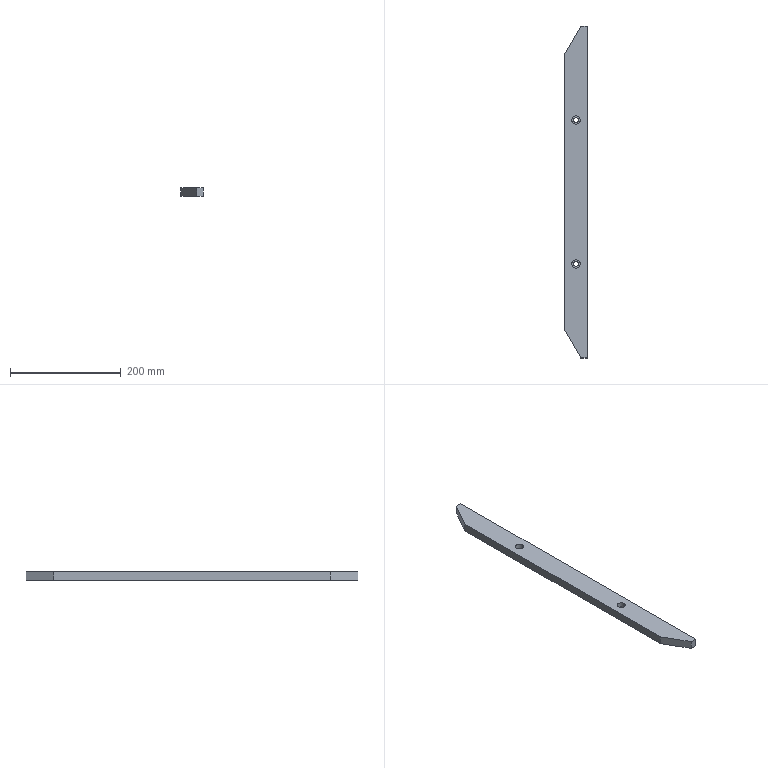Part | SolidWorks | features Chamfer 1, Extrusion 1, HoleWzd 1 | 1 solid | 18 faces | box 40 x 600 x 15 mm | volume 334405 mm3 | plane 10 | cylinder 8 | commonest cylinder face diameters 9 x4 15 x4
STEP:
#1=CARTESIAN_POINT('',(-7.5,-130.,6.));
#2=VERTEX_POINT('',#1);
#3=CARTESIAN_POINT('',(7.5,-130.,6.));
#4=VERTEX_POINT('',#3);
#5=CARTESIAN_POINT('',(0.,-130.,6.));
#6=DIRECTION('',(0.,0.,1.));
#7=DIRECTION('',(1.,0.,0.));
#8=AXIS2_PLACEMENT_3D('',#5,#6,#7);
#9=CIRCLE('',#8,7.5);
#10=EDGE_CURVE('',#2,#4,#9,.T.);
#11=ORIENTED_EDGE('',*,*,#10,.F.);
#12=CARTESIAN_POINT('',(-7.5,-130.,15.));
#13=VERTEX_POINT('',#12);
#14=CARTESIAN_POINT('',(-7.5,-130.,15.));
#15=DIRECTION('',(0.,0.,1.));
#16=VECTOR('',#15,1000.);
#17=LINE('',#14,#16);
#18=EDGE_CURVE('',#2,#13,#17,.T.);
#19=ORIENTED_EDGE('',*,*,#18,.T.);
#20=CARTESIAN_POINT('',(7.5,-130.,15.));
#21=VERTEX_POINT('',#20);
#22=CARTESIAN_POINT('',(0.,-130.,15.));
#23=DIRECTION('',(0.,0.,1.));
#24=DIRECTION('',(1.,0.,0.));
#25=AXIS2_PLACEMENT_3D('',#22,#23,#24);
#26=CIRCLE('',#25,7.5);
#27=EDGE_CURVE('',#13,#21,#26,.T.);
#28=ORIENTED_EDGE('',*,*,#27,.T.);
#29=CARTESIAN_POINT('',(7.5,-130.,15.));
#30=DIRECTION('',(0.,0.,1.));
#31=VECTOR('',#30,1000.);
#32=LINE('',#29,#31);
#33=EDGE_CURVE('',#4,#21,#32,.T.);
#34=ORIENTED_EDGE('',*,*,#33,.F.);
#35=EDGE_LOOP('',(#11,#19,#28,#34));
#36=FACE_OUTER_BOUND('',#35,.T.);
#37=CARTESIAN_POINT('',(0.,-130.,15.));
#38=DIRECTION('',(0.,0.,1.));
#39=DIRECTION('',(1.,0.,0.));
#40=AXIS2_PLACEMENT_3D('',#37,#38,#39);
#41=CYLINDRICAL_SURFACE('',#40,7.5);
#42=ADVANCED_FACE('',(#36),#41,.F.);
#43=CARTESIAN_POINT('',(-4.5,-130.,0.));
#44=VERTEX_POINT('',#43);
#45=CARTESIAN_POINT('',(4.5,-130.,0.));
#46=VERTEX_POINT('',#45);
#47=CARTESIAN_POINT('',(0.,-130.,0.));
#48=DIRECTION('',(0.,0.,1.));
#49=DIRECTION('',(1.,0.,0.));
#50=AXIS2_PLACEMENT_3D('',#47,#48,#49);
#51=CIRCLE('',#50,4.5);
#52=EDGE_CURVE('',#44,#46,#51,.T.);
#53=ORIENTED_EDGE('',*,*,#52,.F.);
#54=CARTESIAN_POINT('',(-4.5,-130.,6.));
#55=VERTEX_POINT('',#54);
#56=CARTESIAN_POINT('',(-4.5,-130.,15.));
#57=DIRECTION('',(0.,0.,1.));
#58=VECTOR('',#57,1000.);
#59=LINE('',#56,#58);
#60=EDGE_CURVE('',#44,#55,#59,.T.);
#61=ORIENTED_EDGE('',*,*,#60,.T.);
#62=CARTESIAN_POINT('',(4.5,-130.,6.));
#63=VERTEX_POINT('',#62);
#64=CARTESIAN_POINT('',(0.,-130.,6.));
#65=DIRECTION('',(0.,0.,1.));
#66=DIRECTION('',(1.,0.,0.));
#67=AXIS2_PLACEMENT_3D('',#64,#65,#66);
#68=CIRCLE('',#67,4.5);
#69=EDGE_CURVE('',#55,#63,#68,.T.);
#70=ORIENTED_EDGE('',*,*,#69,.T.);
#71=CARTESIAN_POINT('',(4.5,-130.,15.));
#72=DIRECTION('',(0.,0.,1.));
#73=VECTOR('',#72,1000.);
#74=LINE('',#71,#73);
#75=EDGE_CURVE('',#46,#63,#74,.T.);
#76=ORIENTED_EDGE('',*,*,#75,.F.);
#77=EDGE_LOOP('',(#53,#61,#70,#76));
#78=FACE_OUTER_BOUND('',#77,.T.);
#79=CARTESIAN_POINT('',(0.,-130.,15.));
#80=DIRECTION('',(0.,0.,1.));
#81=DIRECTION('',(1.,0.,0.));
#82=AXIS2_PLACEMENT_3D('',#79,#80,#81);
#83=CYLINDRICAL_SURFACE('',#82,4.5);
#84=ADVANCED_FACE('',(#78),#83,.F.);
#85=CARTESIAN_POINT('',(-7.5,130.,6.));
#86=VERTEX_POINT('',#85);
#87=CARTESIAN_POINT('',(7.5,130.,6.));
#88=VERTEX_POINT('',#87);
#89=CARTESIAN_POINT('',(0.,130.,6.));
#90=DIRECTION('',(0.,0.,1.));
#91=DIRECTION('',(1.,0.,0.));
#92=AXIS2_PLACEMENT_3D('',#89,#90,#91);
#93=CIRCLE('',#92,7.5);
#94=EDGE_CURVE('',#86,#88,#93,.T.);
#95=ORIENTED_EDGE('',*,*,#94,.F.);
#96=CARTESIAN_POINT('',(-7.5,130.,15.));
#97=VERTEX_POINT('',#96);
#98=CARTESIAN_POINT('',(-7.5,130.,15.));
#99=DIRECTION('',(0.,0.,1.));
#100=VECTOR('',#99,1000.);
#101=LINE('',#98,#100);
#102=EDGE_CURVE('',#86,#97,#101,.T.);
#103=ORIENTED_EDGE('',*,*,#102,.T.);
#104=CARTESIAN_POINT('',(7.5,130.,15.));
#105=VERTEX_POINT('',#104);
#106=CARTESIAN_POINT('',(0.,130.,15.));
#107=DIRECTION('',(0.,0.,1.));
#108=DIRECTION('',(1.,0.,0.));
#109=AXIS2_PLACEMENT_3D('',#106,#107,#108);
#110=CIRCLE('',#109,7.5);
#111=EDGE_CURVE('',#97,#105,#110,.T.);
#112=ORIENTED_EDGE('',*,*,#111,.T.);
#113=CARTESIAN_POINT('',(7.5,130.,15.));
#114=DIRECTION('',(0.,0.,1.));
#115=VECTOR('',#114,1000.);
#116=LINE('',#113,#115);
#117=EDGE_CURVE('',#88,#105,#116,.T.);
#118=ORIENTED_EDGE('',*,*,#117,.F.);
#119=EDGE_LOOP('',(#95,#103,#112,#118));
#120=FACE_OUTER_BOUND('',#119,.T.);
#121=CARTESIAN_POINT('',(0.,130.,15.));
#122=DIRECTION('',(0.,0.,1.));
#123=DIRECTION('',(1.,0.,0.));
#124=AXIS2_PLACEMENT_3D('',#121,#122,#123);
#125=CYLINDRICAL_SURFACE('',#124,7.5);
#126=ADVANCED_FACE('',(#120),#125,.F.);
#127=CARTESIAN_POINT('',(-4.5,130.,0.));
#128=VERTEX_POINT('',#127);
#129=CARTESIAN_POINT('',(4.5,130.,0.));
#130=VERTEX_POINT('',#129);
#131=CARTESIAN_POINT('',(0.,130.,0.));
#132=DIRECTION('',(0.,0.,1.));
#133=DIRECTION('',(1.,0.,0.));
#134=AXIS2_PLACEMENT_3D('',#131,#132,#133);
#135=CIRCLE('',#134,4.5);
#136=EDGE_CURVE('',#128,#130,#135,.T.);
#137=ORIENTED_EDGE('',*,*,#136,.F.);
#138=CARTESIAN_POINT('',(-4.5,130.,6.));
#139=VERTEX_POINT('',#138);
#140=CARTESIAN_POINT('',(-4.5,130.,15.));
#141=DIRECTION('',(0.,0.,1.));
#142=VECTOR('',#141,1000.);
#143=LINE('',#140,#142);
#144=EDGE_CURVE('',#128,#139,#143,.T.);
#145=ORIENTED_EDGE('',*,*,#144,.T.);
#146=CARTESIAN_POINT('',(4.5,130.,6.));
#147=VERTEX_POINT('',#146);
#148=CARTESIAN_POINT('',(0.,130.,6.));
#149=DIRECTION('',(0.,0.,1.));
#150=DIRECTION('',(1.,0.,0.));
#151=AXIS2_PLACEMENT_3D('',#148,#149,#150);
#152=CIRCLE('',#151,4.5);
#153=EDGE_CURVE('',#139,#147,#152,.T.);
#154=ORIENTED_EDGE('',*,*,#153,.T.);
#155=CARTESIAN_POINT('',(4.5,130.,15.));
#156=DIRECTION('',(0.,0.,1.));
#157=VECTOR('',#156,1000.);
#158=LINE('',#155,#157);
#159=EDGE_CURVE('',#130,#147,#158,.T.);
#160=ORIENTED_EDGE('',*,*,#159,.F.);
#161=EDGE_LOOP('',(#137,#145,#154,#160));
#162=FACE_OUTER_BOUND('',#161,.T.);
#163=CARTESIAN_POINT('',(0.,130.,15.));
#164=DIRECTION('',(0.,0.,1.));
#165=DIRECTION('',(1.,0.,0.));
#166=AXIS2_PLACEMENT_3D('',#163,#164,#165);
#167=CYLINDRICAL_SURFACE('',#166,4.5);
#168=ADVANCED_FACE('',(#162),#167,.F.);
#169=CARTESIAN_POINT('',(-20.,250.,15.));
#170=VERTEX_POINT('',#169);
#171=CARTESIAN_POINT('',(-20.,-250.,15.));
#172=VERTEX_POINT('',#171);
#173=CARTESIAN_POINT('',(-20.,-300.,15.));
#174=DIRECTION('',(0.,-1.,0.));
#175=VECTOR('',#174,1000.);
#176=LINE('',#173,#175);
#177=EDGE_CURVE('',#170,#172,#176,.T.);
#178=ORIENTED_EDGE('',*,*,#177,.F.);
#179=CARTESIAN_POINT('',(-20.,250.,0.));
#180=VERTEX_POINT('',#179);
#181=CARTESIAN_POINT('',(-20.,250.,15.));
#182=DIRECTION('',(0.,0.,-1.));
#183=VECTOR('',#182,1000.);
#184=LINE('',#181,#183);
#185=EDGE_CURVE('',#170,#180,#184,.T.);
#186=ORIENTED_EDGE('',*,*,#185,.T.);
#187=CARTESIAN_POINT('',(-20.,-250.,0.));
#188=VERTEX_POINT('',#187);
#189=CARTESIAN_POINT('',(-20.,-300.,0.));
#190=DIRECTION('',(0.,-1.,0.));
#191=VECTOR('',#190,1000.);
#192=LINE('',#189,#191);
#193=EDGE_CURVE('',#180,#188,#192,.T.);
#194=ORIENTED_EDGE('',*,*,#193,.T.);
#195=CARTESIAN_POINT('',(-20.,-250.,15.));
#196=DIRECTION('',(0.,0.,1.));
#197=VECTOR('',#196,1000.);
#198=LINE('',#195,#197);
#199=EDGE_CURVE('',#188,#172,#198,.T.);
#200=ORIENTED_EDGE('',*,*,#199,.T.);
#201=EDGE_LOOP('',(#178,#186,#194,#200));
#202=FACE_OUTER_BOUND('',#201,.T.);
#203=CARTESIAN_POINT('',(-20.,-300.,15.));
#204=DIRECTION('',(1.,0.,0.));
#205=DIRECTION('',(0.,0.,-1.));
#206=AXIS2_PLACEMENT_3D('',#203,#204,#205);
#207=PLANE('',#206);
#208=ADVANCED_FACE('',(#202),#207,.F.);
#209=CARTESIAN_POINT('',(8.868,-300.,15.));
#210=VERTEX_POINT('',#209);
#211=CARTESIAN_POINT('',(20.,-300.,15.));
#212=VERTEX_POINT('',#211);
#213=CARTESIAN_POINT('',(20.,-300.,15.));
#214=DIRECTION('',(1.,0.,0.));
#215=VECTOR('',#214,1000.);
#216=LINE('',#213,#215);
#217=EDGE_CURVE('',#210,#212,#216,.T.);
#218=ORIENTED_EDGE('',*,*,#217,.F.);
#219=CARTESIAN_POINT('',(8.868,-300.,0.));
#220=VERTEX_POINT('',#219);
#221=CARTESIAN_POINT('',(8.868,-300.,15.));
#222=DIRECTION('',(0.,0.,-1.));
#223=VECTOR('',#222,1000.);
#224=LINE('',#221,#223);
#225=EDGE_CURVE('',#210,#220,#224,.T.);
#226=ORIENTED_EDGE('',*,*,#225,.T.);
#227=CARTESIAN_POINT('',(20.,-300.,0.));
#228=VERTEX_POINT('',#227);
#229=CARTESIAN_POINT('',(20.,-300.,0.));
#230=DIRECTION('',(1.,0.,0.));
#231=VECTOR('',#230,1000.);
#232=LINE('',#229,#231);
#233=EDGE_CURVE('',#220,#228,#232,.T.);
#234=ORIENTED_EDGE('',*,*,#233,.T.);
#235=CARTESIAN_POINT('',(20.,-300.,15.));
#236=DIRECTION('',(0.,0.,-1.));
#237=VECTOR('',#236,1000.);
#238=LINE('',#235,#237);
#239=EDGE_CURVE('',#212,#228,#238,.T.);
#240=ORIENTED_EDGE('',*,*,#239,.F.);
#241=EDGE_LOOP('',(#218,#226,#234,#240));
#242=FACE_OUTER_BOUND('',#241,.T.);
#243=CARTESIAN_POINT('',(20.,-300.,15.));
#244=DIRECTION('',(0.,1.,0.));
#245=DIRECTION('',(0.,0.,1.));
#246=AXIS2_PLACEMENT_3D('',#243,#244,#245);
#247=PLANE('',#246);
#248=ADVANCED_FACE('',(#242),#247,.F.);
#249=CARTESIAN_POINT('',(20.,300.,0.));
#250=VERTEX_POINT('',#249);
#251=CARTESIAN_POINT('',(20.,-300.,0.));
#252=DIRECTION('',(0.,1.,0.));
#253=VECTOR('',#252,1000.);
#254=LINE('',#251,#253);
#255=EDGE_CURVE('',#228,#250,#254,.T.);
#256=ORIENTED_EDGE('',*,*,#255,.T.);
#257=CARTESIAN_POINT('',(20.,300.,15.));
#258=VERTEX_POINT('',#257);
#259=CARTESIAN_POINT('',(20.,300.,15.));
#260=DIRECTION('',(0.,0.,-1.));
#261=VECTOR('',#260,1000.);
#262=LINE('',#259,#261);
#263=EDGE_CURVE('',#258,#250,#262,.T.);
#264=ORIENTED_EDGE('',*,*,#263,.F.);
#265=CARTESIAN_POINT('',(20.,-300.,15.));
#266=DIRECTION('',(0.,1.,0.));
#267=VECTOR('',#266,1000.);
#268=LINE('',#265,#267);
#269=EDGE_CURVE('',#212,#258,#268,.T.);
#270=ORIENTED_EDGE('',*,*,#269,.F.);
#271=ORIENTED_EDGE('',*,*,#239,.T.);
#272=EDGE_LOOP('',(#256,#264,#270,#271));
#273=FACE_OUTER_BOUND('',#272,.T.);
#274=CARTESIAN_POINT('',(20.,-300.,15.));
#275=DIRECTION('',(-1.,0.,0.));
#276=DIRECTION('',(0.,0.,1.));
#277=AXIS2_PLACEMENT_3D('',#274,#275,#276);
#278=PLANE('',#277);
#279=ADVANCED_FACE('',(#273),#278,.F.);
#280=CARTESIAN_POINT('',(8.868,300.,0.));
#281=VERTEX_POINT('',#280);
#282=CARTESIAN_POINT('',(20.,300.,0.));
#283=DIRECTION('',(-1.,0.,0.));
#284=VECTOR('',#283,1000.);
#285=LINE('',#282,#284);
#286=EDGE_CURVE('',#250,#281,#285,.T.);
#287=ORIENTED_EDGE('',*,*,#286,.T.);
#288=CARTESIAN_POINT('',(8.868,300.,15.));
#289=VERTEX_POINT('',#288);
#290=CARTESIAN_POINT('',(8.868,300.,15.));
#291=DIRECTION('',(0.,0.,1.));
#292=VECTOR('',#291,1000.);
#293=LINE('',#290,#292);
#294=EDGE_CURVE('',#281,#289,#293,.T.);
#295=ORIENTED_EDGE('',*,*,#294,.T.);
#296=CARTESIAN_POINT('',(20.,300.,15.));
#297=DIRECTION('',(-1.,0.,0.));
#298=VECTOR('',#297,1000.);
#299=LINE('',#296,#298);
#300=EDGE_CURVE('',#258,#289,#299,.T.);
#301=ORIENTED_EDGE('',*,*,#300,.F.);
#302=ORIENTED_EDGE('',*,*,#263,.T.);
#303=EDGE_LOOP('',(#287,#295,#301,#302));
#304=FACE_OUTER_BOUND('',#303,.T.);
#305=CARTESIAN_POINT('',(20.,300.,15.));
#306=DIRECTION('',(0.,-1.,0.));
#307=DIRECTION('',(0.,0.,-1.));
#308=AXIS2_PLACEMENT_3D('',#305,#306,#307);
#309=PLANE('',#308);
#310=ADVANCED_FACE('',(#304),#309,.F.);
#311=CARTESIAN_POINT('',(0.,-130.,15.));
#312=DIRECTION('',(0.,0.,1.));
#313=DIRECTION('',(1.,0.,0.));
#314=AXIS2_PLACEMENT_3D('',#311,#312,#313);
#315=CIRCLE('',#314,7.5);
#316=EDGE_CURVE('',#21,#13,#315,.T.);
#317=ORIENTED_EDGE('',*,*,#316,.F.);
#318=ORIENTED_EDGE('',*,*,#27,.F.);
#319=EDGE_LOOP('',(#317,#318));
#320=FACE_BOUND('',#319,.T.);
#321=CARTESIAN_POINT('',(0.,130.,15.));
#322=DIRECTION('',(0.,0.,1.));
#323=DIRECTION('',(1.,0.,0.));
#324=AXIS2_PLACEMENT_3D('',#321,#322,#323);
#325=CIRCLE('',#324,7.5);
#326=EDGE_CURVE('',#105,#97,#325,.T.);
#327=ORIENTED_EDGE('',*,*,#326,.F.);
#328=ORIENTED_EDGE('',*,*,#111,.F.);
#329=EDGE_LOOP('',(#327,#328));
#330=FACE_BOUND('',#329,.T.);
#331=ORIENTED_EDGE('',*,*,#300,.T.);
#332=CARTESIAN_POINT('',(-123.253,71.16,15.));
#333=DIRECTION('',(-0.5,-0.866,0.));
#334=VECTOR('',#333,1000.);
#335=LINE('',#332,#334);
#336=EDGE_CURVE('',#289,#170,#335,.T.);
#337=ORIENTED_EDGE('',*,*,#336,.T.);
#338=ORIENTED_EDGE('',*,*,#177,.T.);
#339=CARTESIAN_POINT('',(-123.253,-71.16,15.));
#340=DIRECTION('',(0.5,-0.866,0.));
#341=VECTOR('',#340,1000.);
#342=LINE('',#339,#341);
#343=EDGE_CURVE('',#172,#210,#342,.T.);
#344=ORIENTED_EDGE('',*,*,#343,.T.);
#345=ORIENTED_EDGE('',*,*,#217,.T.);
#346=ORIENTED_EDGE('',*,*,#269,.T.);
#347=EDGE_LOOP('',(#331,#337,#338,#344,#345,#346));
#348=FACE_OUTER_BOUND('',#347,.T.);
#349=CARTESIAN_POINT('',(0.,0.,15.));
#350=DIRECTION('',(0.,0.,1.));
#351=DIRECTION('',(1.,0.,0.));
#352=AXIS2_PLACEMENT_3D('',#349,#350,#351);
#353=PLANE('',#352);
#354=ADVANCED_FACE('',(#320,#330,#348),#353,.T.);
#355=CARTESIAN_POINT('',(0.,-130.,0.));
#356=DIRECTION('',(0.,0.,1.));
#357=DIRECTION('',(1.,0.,0.));
#358=AXIS2_PLACEMENT_3D('',#355,#356,#357);
#359=CIRCLE('',#358,4.5);
#360=EDGE_CURVE('',#46,#44,#359,.T.);
#361=ORIENTED_EDGE('',*,*,#360,.T.);
#362=ORIENTED_EDGE('',*,*,#52,.T.);
#363=EDGE_LOOP('',(#361,#362));
#364=FACE_BOUND('',#363,.T.);
#365=CARTESIAN_POINT('',(0.,130.,0.));
#366=DIRECTION('',(0.,0.,1.));
#367=DIRECTION('',(1.,0.,0.));
#368=AXIS2_PLACEMENT_3D('',#365,#366,#367);
#369=CIRCLE('',#368,4.5);
#370=EDGE_CURVE('',#130,#128,#369,.T.);
#371=ORIENTED_EDGE('',*,*,#370,.T.);
#372=ORIENTED_EDGE('',*,*,#136,.T.);
#373=EDGE_LOOP('',(#371,#372));
#374=FACE_BOUND('',#373,.T.);
#375=ORIENTED_EDGE('',*,*,#193,.F.);
#376=CARTESIAN_POINT('',(-20.,250.,0.));
#377=DIRECTION('',(0.5,0.866,0.));
#378=VECTOR('',#377,1000.);
#379=LINE('',#376,#378);
#380=EDGE_CURVE('',#180,#281,#379,.T.);
#381=ORIENTED_EDGE('',*,*,#380,.T.);
#382=ORIENTED_EDGE('',*,*,#286,.F.);
#383=ORIENTED_EDGE('',*,*,#255,.F.);
#384=ORIENTED_EDGE('',*,*,#233,.F.);
#385=CARTESIAN_POINT('',(8.868,-300.,0.));
#386=DIRECTION('',(-0.5,0.866,0.));
#387=VECTOR('',#386,1000.);
#388=LINE('',#385,#387);
#389=EDGE_CURVE('',#220,#188,#388,.T.);
#390=ORIENTED_EDGE('',*,*,#389,.T.);
#391=EDGE_LOOP('',(#375,#381,#382,#383,#384,#390));
#392=FACE_OUTER_BOUND('',#391,.T.);
#393=CARTESIAN_POINT('',(0.,0.,0.));
#394=DIRECTION('',(0.,0.,1.));
#395=DIRECTION('',(1.,0.,0.));
#396=AXIS2_PLACEMENT_3D('',#393,#394,#395);
#397=PLANE('',#396);
#398=ADVANCED_FACE('',(#364,#374,#392),#397,.F.);
#399=ORIENTED_EDGE('',*,*,#144,.F.);
#400=ORIENTED_EDGE('',*,*,#370,.F.);
#401=ORIENTED_EDGE('',*,*,#159,.T.);
#402=CARTESIAN_POINT('',(0.,130.,6.));
#403=DIRECTION('',(0.,0.,1.));
#404=DIRECTION('',(1.,0.,0.));
#405=AXIS2_PLACEMENT_3D('',#402,#403,#404);
#406=CIRCLE('',#405,4.5);
#407=EDGE_CURVE('',#147,#139,#406,.T.);
#408=ORIENTED_EDGE('',*,*,#407,.T.);
#409=EDGE_LOOP('',(#399,#400,#401,#408));
#410=FACE_OUTER_BOUND('',#409,.T.);
#411=CARTESIAN_POINT('',(0.,130.,15.));
#412=DIRECTION('',(0.,0.,1.));
#413=DIRECTION('',(1.,0.,0.));
#414=AXIS2_PLACEMENT_3D('',#411,#412,#413);
#415=CYLINDRICAL_SURFACE('',#414,4.5);
#416=ADVANCED_FACE('',(#410),#415,.F.);
#417=ORIENTED_EDGE('',*,*,#407,.F.);
#418=ORIENTED_EDGE('',*,*,#153,.F.);
#419=EDGE_LOOP('',(#417,#418));
#420=FACE_BOUND('',#419,.T.);
#421=CARTESIAN_POINT('',(0.,130.,6.));
#422=DIRECTION('',(0.,0.,1.));
#423=DIRECTION('',(1.,0.,0.));
#424=AXIS2_PLACEMENT_3D('',#421,#422,#423);
#425=CIRCLE('',#424,7.5);
#426=EDGE_CURVE('',#88,#86,#425,.T.);
#427=ORIENTED_EDGE('',*,*,#426,.T.);
#428=ORIENTED_EDGE('',*,*,#94,.T.);
#429=EDGE_LOOP('',(#427,#428));
#430=FACE_OUTER_BOUND('',#429,.T.);
#431=CARTESIAN_POINT('',(4.5,130.,6.));
#432=DIRECTION('',(0.,0.,-1.));
#433=DIRECTION('',(-1.,0.,0.));
#434=AXIS2_PLACEMENT_3D('',#431,#432,#433);
#435=PLANE('',#434);
#436=ADVANCED_FACE('',(#420,#430),#435,.F.);
#437=ORIENTED_EDGE('',*,*,#102,.F.);
#438=ORIENTED_EDGE('',*,*,#426,.F.);
#439=ORIENTED_EDGE('',*,*,#117,.T.);
#440=ORIENTED_EDGE('',*,*,#326,.T.);
#441=EDGE_LOOP('',(#437,#438,#439,#440));
#442=FACE_OUTER_BOUND('',#441,.T.);
#443=CARTESIAN_POINT('',(0.,130.,15.));
#444=DIRECTION('',(0.,0.,1.));
#445=DIRECTION('',(1.,0.,0.));
#446=AXIS2_PLACEMENT_3D('',#443,#444,#445);
#447=CYLINDRICAL_SURFACE('',#446,7.5);
#448=ADVANCED_FACE('',(#442),#447,.F.);
#449=ORIENTED_EDGE('',*,*,#60,.F.);
#450=ORIENTED_EDGE('',*,*,#360,.F.);
#451=ORIENTED_EDGE('',*,*,#75,.T.);
#452=CARTESIAN_POINT('',(0.,-130.,6.));
#453=DIRECTION('',(0.,0.,1.));
#454=DIRECTION('',(1.,0.,0.));
#455=AXIS2_PLACEMENT_3D('',#452,#453,#454);
#456=CIRCLE('',#455,4.5);
#457=EDGE_CURVE('',#63,#55,#456,.T.);
#458=ORIENTED_EDGE('',*,*,#457,.T.);
#459=EDGE_LOOP('',(#449,#450,#451,#458));
#460=FACE_OUTER_BOUND('',#459,.T.);
#461=CARTESIAN_POINT('',(0.,-130.,15.));
#462=DIRECTION('',(0.,0.,1.));
#463=DIRECTION('',(1.,0.,0.));
#464=AXIS2_PLACEMENT_3D('',#461,#462,#463);
#465=CYLINDRICAL_SURFACE('',#464,4.5);
#466=ADVANCED_FACE('',(#460),#465,.F.);
#467=ORIENTED_EDGE('',*,*,#457,.F.);
#468=ORIENTED_EDGE('',*,*,#69,.F.);
#469=EDGE_LOOP('',(#467,#468));
#470=FACE_BOUND('',#469,.T.);
#471=CARTESIAN_POINT('',(0.,-130.,6.));
#472=DIRECTION('',(0.,0.,1.));
#473=DIRECTION('',(1.,0.,0.));
#474=AXIS2_PLACEMENT_3D('',#471,#472,#473);
#475=CIRCLE('',#474,7.5);
#476=EDGE_CURVE('',#4,#2,#475,.T.);
#477=ORIENTED_EDGE('',*,*,#476,.T.);
#478=ORIENTED_EDGE('',*,*,#10,.T.);
#479=EDGE_LOOP('',(#477,#478));
#480=FACE_OUTER_BOUND('',#479,.T.);
#481=CARTESIAN_POINT('',(4.5,-130.,6.));
#482=DIRECTION('',(0.,0.,-1.));
#483=DIRECTION('',(-1.,0.,0.));
#484=AXIS2_PLACEMENT_3D('',#481,#482,#483);
#485=PLANE('',#484);
#486=ADVANCED_FACE('',(#470,#480),#485,.F.);
#487=ORIENTED_EDGE('',*,*,#18,.F.);
#488=ORIENTED_EDGE('',*,*,#476,.F.);
#489=ORIENTED_EDGE('',*,*,#33,.T.);
#490=ORIENTED_EDGE('',*,*,#316,.T.);
#491=EDGE_LOOP('',(#487,#488,#489,#490));
#492=FACE_OUTER_BOUND('',#491,.T.);
#493=CARTESIAN_POINT('',(0.,-130.,15.));
#494=DIRECTION('',(0.,0.,1.));
#495=DIRECTION('',(1.,0.,0.));
#496=AXIS2_PLACEMENT_3D('',#493,#494,#495);
#497=CYLINDRICAL_SURFACE('',#496,7.5);
#498=ADVANCED_FACE('',(#492),#497,.F.);
#499=ORIENTED_EDGE('',*,*,#336,.F.);
#500=ORIENTED_EDGE('',*,*,#294,.F.);
#501=ORIENTED_EDGE('',*,*,#380,.F.);
#502=ORIENTED_EDGE('',*,*,#185,.F.);
#503=EDGE_LOOP('',(#499,#500,#501,#502));
#504=FACE_OUTER_BOUND('',#503,.T.);
#505=CARTESIAN_POINT('',(-20.,250.,15.));
#506=DIRECTION('',(0.866,-0.5,0.));
#507=DIRECTION('',(0.,0.,-1.));
#508=AXIS2_PLACEMENT_3D('',#505,#506,#507);
#509=PLANE('',#508);
#510=ADVANCED_FACE('',(#504),#509,.F.);
#511=ORIENTED_EDGE('',*,*,#343,.F.);
#512=ORIENTED_EDGE('',*,*,#199,.F.);
#513=ORIENTED_EDGE('',*,*,#389,.F.);
#514=ORIENTED_EDGE('',*,*,#225,.F.);
#515=EDGE_LOOP('',(#511,#512,#513,#514));
#516=FACE_OUTER_BOUND('',#515,.T.);
#517=CARTESIAN_POINT('',(8.868,-300.,15.));
#518=DIRECTION('',(0.866,0.5,0.));
#519=DIRECTION('',(0.,0.,-1.));
#520=AXIS2_PLACEMENT_3D('',#517,#518,#519);
#521=PLANE('',#520);
#522=ADVANCED_FACE('',(#516),#521,.F.);
#523=CLOSED_SHELL('',(#42,#84,#126,#168,#208,#248,#279,#310,#354,#398,#416,#436,#448,#466,#486,#498,#510,#522));
#524=MANIFOLD_SOLID_BREP('',#523);
#525=CARTESIAN_POINT('',(0.,0.,0.));
#526=DIRECTION('',(0.,0.,1.));
#527=DIRECTION('',(1.,0.,0.));
#528=AXIS2_PLACEMENT_3D('',#525,#526,#527);
#529=(LENGTH_UNIT()NAMED_UNIT(*)SI_UNIT(.MILLI.,.METRE.));
#530=UNCERTAINTY_MEASURE_WITH_UNIT(LENGTH_MEASURE(0.00001),#529,'','');
#531=(NAMED_UNIT(*)PLANE_ANGLE_UNIT()SI_UNIT($,.RADIAN.));
#532=(NAMED_UNIT(*)SI_UNIT($,.STERADIAN.)SOLID_ANGLE_UNIT());
#533=(GEOMETRIC_REPRESENTATION_CONTEXT(3)GLOBAL_UNCERTAINTY_ASSIGNED_CONTEXT((#530))GLOBAL_UNIT_ASSIGNED_CONTEXT((#529,#531,#532))REPRESENTATION_CONTEXT('',''));
#534=ADVANCED_BREP_SHAPE_REPRESENTATION('',(#524,#528),#533);